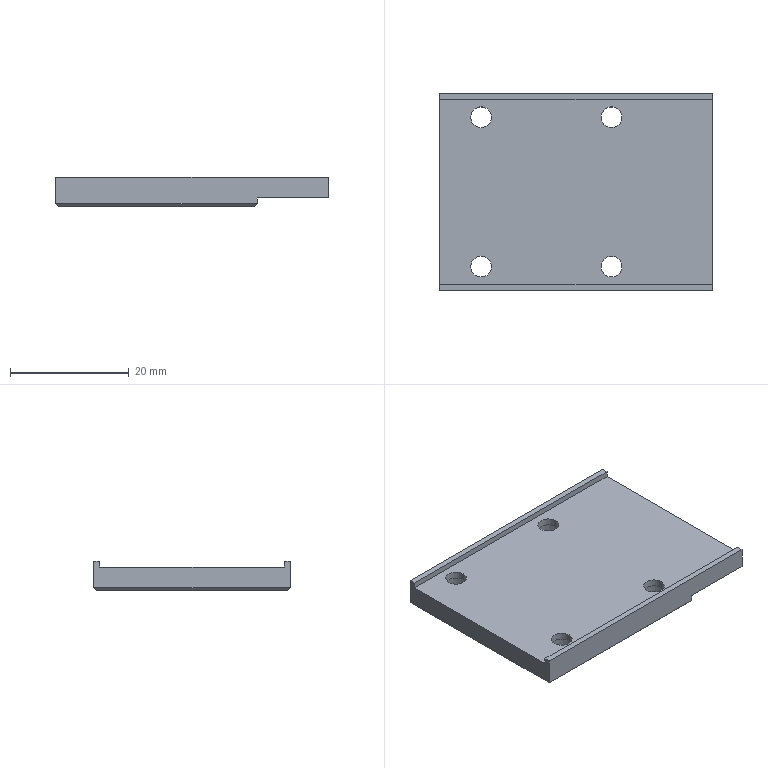Part | NX | 1 solid | 36 faces | box 46 x 33.2 x 5 mm | volume 5224 mm3 | plane 20 | cylinder 16 | commonest cylinder face diameters 3.5 x8 6 x8
STEP:
#1=CARTESIAN_POINT('',(0.,-32.2,4.5));
#2=VERTEX_POINT('',#1);
#3=CARTESIAN_POINT('',(46.,-32.2,4.5));
#4=VERTEX_POINT('',#3);
#5=CARTESIAN_POINT('',(0.,-32.2,4.5));
#6=DIRECTION('',(1.,0.,0.));
#7=VECTOR('',#6,1000.);
#8=LINE('',#5,#7);
#9=EDGE_CURVE('',#2,#4,#8,.T.);
#10=ORIENTED_EDGE('',*,*,#9,.T.);
#11=CARTESIAN_POINT('',(46.,-1.,4.5));
#12=VERTEX_POINT('',#11);
#13=CARTESIAN_POINT('',(46.,0.,4.5));
#14=DIRECTION('',(0.,-1.,0.));
#15=VECTOR('',#14,1000.);
#16=LINE('',#13,#15);
#17=EDGE_CURVE('',#12,#4,#16,.T.);
#18=ORIENTED_EDGE('',*,*,#17,.F.);
#19=CARTESIAN_POINT('',(0.,-1.,4.5));
#20=VERTEX_POINT('',#19);
#21=CARTESIAN_POINT('',(0.,-1.,4.5));
#22=DIRECTION('',(-1.,0.,0.));
#23=VECTOR('',#22,1000.);
#24=LINE('',#21,#23);
#25=EDGE_CURVE('',#12,#20,#24,.T.);
#26=ORIENTED_EDGE('',*,*,#25,.T.);
#27=CARTESIAN_POINT('',(0.,0.,4.5));
#28=DIRECTION('',(0.,1.,0.));
#29=VECTOR('',#28,1000.);
#30=LINE('',#27,#29);
#31=EDGE_CURVE('',#2,#20,#30,.T.);
#32=ORIENTED_EDGE('',*,*,#31,.F.);
#33=EDGE_LOOP('',(#10,#18,#26,#32));
#34=FACE_BOUND('',#33,.T.);
#35=CARTESIAN_POINT('',(8.75,-29.2,4.5));
#36=VERTEX_POINT('',#35);
#37=CARTESIAN_POINT('',(5.25,-29.2,4.5));
#38=VERTEX_POINT('',#37);
#39=CARTESIAN_POINT('',(7.,-29.2,4.5));
#40=DIRECTION('',(0.,0.,-1.));
#41=DIRECTION('',(1.,0.,0.));
#42=AXIS2_PLACEMENT_3D('',#39,#40,#41);
#43=CIRCLE('',#42,1.75);
#44=EDGE_CURVE('',#36,#38,#43,.T.);
#45=ORIENTED_EDGE('',*,*,#44,.T.);
#46=CARTESIAN_POINT('',(7.,-29.2,4.5));
#47=DIRECTION('',(0.,0.,-1.));
#48=DIRECTION('',(1.,0.,0.));
#49=AXIS2_PLACEMENT_3D('',#46,#47,#48);
#50=CIRCLE('',#49,1.75);
#51=EDGE_CURVE('',#38,#36,#50,.T.);
#52=ORIENTED_EDGE('',*,*,#51,.T.);
#53=EDGE_LOOP('',(#45,#52));
#54=FACE_BOUND('',#53,.T.);
#55=CARTESIAN_POINT('',(30.75,-4.,4.5));
#56=VERTEX_POINT('',#55);
#57=CARTESIAN_POINT('',(27.25,-4.,4.5));
#58=VERTEX_POINT('',#57);
#59=CARTESIAN_POINT('',(29.,-4.,4.5));
#60=DIRECTION('',(0.,0.,-1.));
#61=DIRECTION('',(1.,0.,0.));
#62=AXIS2_PLACEMENT_3D('',#59,#60,#61);
#63=CIRCLE('',#62,1.75);
#64=EDGE_CURVE('',#56,#58,#63,.T.);
#65=ORIENTED_EDGE('',*,*,#64,.T.);
#66=CARTESIAN_POINT('',(29.,-4.,4.5));
#67=DIRECTION('',(0.,0.,-1.));
#68=DIRECTION('',(1.,0.,0.));
#69=AXIS2_PLACEMENT_3D('',#66,#67,#68);
#70=CIRCLE('',#69,1.75);
#71=EDGE_CURVE('',#58,#56,#70,.T.);
#72=ORIENTED_EDGE('',*,*,#71,.T.);
#73=EDGE_LOOP('',(#65,#72));
#74=FACE_BOUND('',#73,.T.);
#75=CARTESIAN_POINT('',(27.25,-29.2,4.5));
#76=VERTEX_POINT('',#75);
#77=CARTESIAN_POINT('',(30.75,-29.2,4.5));
#78=VERTEX_POINT('',#77);
#79=CARTESIAN_POINT('',(29.,-29.2,4.5));
#80=DIRECTION('',(0.,0.,-1.));
#81=DIRECTION('',(1.,0.,0.));
#82=AXIS2_PLACEMENT_3D('',#79,#80,#81);
#83=CIRCLE('',#82,1.75);
#84=EDGE_CURVE('',#76,#78,#83,.T.);
#85=ORIENTED_EDGE('',*,*,#84,.T.);
#86=CARTESIAN_POINT('',(29.,-29.2,4.5));
#87=DIRECTION('',(0.,0.,-1.));
#88=DIRECTION('',(1.,0.,0.));
#89=AXIS2_PLACEMENT_3D('',#86,#87,#88);
#90=CIRCLE('',#89,1.75);
#91=EDGE_CURVE('',#78,#76,#90,.T.);
#92=ORIENTED_EDGE('',*,*,#91,.T.);
#93=EDGE_LOOP('',(#85,#92));
#94=FACE_BOUND('',#93,.T.);
#95=CARTESIAN_POINT('',(8.75,-4.,4.5));
#96=VERTEX_POINT('',#95);
#97=CARTESIAN_POINT('',(5.25,-4.,4.5));
#98=VERTEX_POINT('',#97);
#99=CARTESIAN_POINT('',(7.,-4.,4.5));
#100=DIRECTION('',(0.,0.,-1.));
#101=DIRECTION('',(1.,0.,0.));
#102=AXIS2_PLACEMENT_3D('',#99,#100,#101);
#103=CIRCLE('',#102,1.75);
#104=EDGE_CURVE('',#96,#98,#103,.T.);
#105=ORIENTED_EDGE('',*,*,#104,.T.);
#106=CARTESIAN_POINT('',(7.,-4.,4.5));
#107=DIRECTION('',(0.,0.,-1.));
#108=DIRECTION('',(1.,0.,0.));
#109=AXIS2_PLACEMENT_3D('',#106,#107,#108);
#110=CIRCLE('',#109,1.75);
#111=EDGE_CURVE('',#98,#96,#110,.T.);
#112=ORIENTED_EDGE('',*,*,#111,.T.);
#113=EDGE_LOOP('',(#105,#112));
#114=FACE_BOUND('',#113,.T.);
#115=CARTESIAN_POINT('',(0.,0.,4.5));
#116=DIRECTION('',(0.,0.,1.));
#117=DIRECTION('',(1.,0.,0.));
#118=AXIS2_PLACEMENT_3D('',#115,#116,#117);
#119=PLANE('',#118);
#120=ADVANCED_FACE('',(#34,#54,#74,#94,#114),#119,.T.);
#121=CARTESIAN_POINT('',(34.,0.,1.));
#122=VERTEX_POINT('',#121);
#123=CARTESIAN_POINT('',(34.,-33.2,1.));
#124=VERTEX_POINT('',#123);
#125=CARTESIAN_POINT('',(34.,0.,1.));
#126=DIRECTION('',(0.,-1.,0.));
#127=VECTOR('',#126,1000.);
#128=LINE('',#125,#127);
#129=EDGE_CURVE('',#122,#124,#128,.T.);
#130=ORIENTED_EDGE('',*,*,#129,.F.);
#131=CARTESIAN_POINT('',(34.,0.,2.));
#132=VERTEX_POINT('',#131);
#133=CARTESIAN_POINT('',(34.,0.,0.));
#134=DIRECTION('',(0.,0.,1.));
#135=VECTOR('',#134,1000.);
#136=LINE('',#133,#135);
#137=EDGE_CURVE('',#122,#132,#136,.T.);
#138=ORIENTED_EDGE('',*,*,#137,.T.);
#139=CARTESIAN_POINT('',(34.,-33.2,2.));
#140=VERTEX_POINT('',#139);
#141=CARTESIAN_POINT('',(34.,0.,2.));
#142=DIRECTION('',(0.,-1.,0.));
#143=VECTOR('',#142,1000.);
#144=LINE('',#141,#143);
#145=EDGE_CURVE('',#132,#140,#144,.T.);
#146=ORIENTED_EDGE('',*,*,#145,.T.);
#147=CARTESIAN_POINT('',(34.,-33.2,0.));
#148=DIRECTION('',(0.,0.,1.));
#149=VECTOR('',#148,1000.);
#150=LINE('',#147,#149);
#151=EDGE_CURVE('',#124,#140,#150,.T.);
#152=ORIENTED_EDGE('',*,*,#151,.F.);
#153=EDGE_LOOP('',(#130,#138,#146,#152));
#154=FACE_BOUND('',#153,.T.);
#155=CARTESIAN_POINT('',(34.,0.,0.));
#156=DIRECTION('',(-1.,0.,0.));
#157=DIRECTION('',(0.,0.,1.));
#158=AXIS2_PLACEMENT_3D('',#155,#156,#157);
#159=PLANE('',#158);
#160=ADVANCED_FACE('',(#154),#159,.F.);
#161=CARTESIAN_POINT('',(0.,-33.2,5.5));
#162=VERTEX_POINT('',#161);
#163=CARTESIAN_POINT('',(0.,-33.2,1.));
#164=VERTEX_POINT('',#163);
#165=CARTESIAN_POINT('',(0.,-33.2,0.));
#166=DIRECTION('',(0.,0.,-1.));
#167=VECTOR('',#166,1000.);
#168=LINE('',#165,#167);
#169=EDGE_CURVE('',#162,#164,#168,.T.);
#170=ORIENTED_EDGE('',*,*,#169,.T.);
#171=CARTESIAN_POINT('',(0.,-33.2,1.));
#172=DIRECTION('',(1.,0.,0.));
#173=VECTOR('',#172,1000.);
#174=LINE('',#171,#173);
#175=EDGE_CURVE('',#164,#124,#174,.T.);
#176=ORIENTED_EDGE('',*,*,#175,.T.);
#177=ORIENTED_EDGE('',*,*,#151,.T.);
#178=CARTESIAN_POINT('',(46.,-33.2,2.));
#179=VERTEX_POINT('',#178);
#180=CARTESIAN_POINT('',(0.,-33.2,2.));
#181=DIRECTION('',(1.,0.,0.));
#182=VECTOR('',#181,1000.);
#183=LINE('',#180,#182);
#184=EDGE_CURVE('',#140,#179,#183,.T.);
#185=ORIENTED_EDGE('',*,*,#184,.T.);
#186=CARTESIAN_POINT('',(46.,-33.2,5.5));
#187=VERTEX_POINT('',#186);
#188=CARTESIAN_POINT('',(46.,-33.2,0.));
#189=DIRECTION('',(0.,0.,-1.));
#190=VECTOR('',#189,1000.);
#191=LINE('',#188,#190);
#192=EDGE_CURVE('',#187,#179,#191,.T.);
#193=ORIENTED_EDGE('',*,*,#192,.F.);
#194=CARTESIAN_POINT('',(0.,-33.2,5.5));
#195=DIRECTION('',(1.,0.,0.));
#196=VECTOR('',#195,1000.);
#197=LINE('',#194,#196);
#198=EDGE_CURVE('',#162,#187,#197,.T.);
#199=ORIENTED_EDGE('',*,*,#198,.F.);
#200=EDGE_LOOP('',(#170,#176,#177,#185,#193,#199));
#201=FACE_BOUND('',#200,.T.);
#202=CARTESIAN_POINT('',(0.,-33.2,0.));
#203=DIRECTION('',(0.,-1.,0.));
#204=DIRECTION('',(0.,0.,-1.));
#205=AXIS2_PLACEMENT_3D('',#202,#203,#204);
#206=PLANE('',#205);
#207=ADVANCED_FACE('',(#201),#206,.T.);
#208=CARTESIAN_POINT('',(0.,0.,1.));
#209=VERTEX_POINT('',#208);
#210=CARTESIAN_POINT('',(0.,0.,5.5));
#211=VERTEX_POINT('',#210);
#212=CARTESIAN_POINT('',(0.,0.,0.));
#213=DIRECTION('',(0.,0.,1.));
#214=VECTOR('',#213,1000.);
#215=LINE('',#212,#214);
#216=EDGE_CURVE('',#209,#211,#215,.T.);
#217=ORIENTED_EDGE('',*,*,#216,.F.);
#218=CARTESIAN_POINT('',(0.,0.,1.));
#219=DIRECTION('',(0.,-1.,0.));
#220=VECTOR('',#219,1000.);
#221=LINE('',#218,#220);
#222=EDGE_CURVE('',#209,#164,#221,.T.);
#223=ORIENTED_EDGE('',*,*,#222,.T.);
#224=ORIENTED_EDGE('',*,*,#169,.F.);
#225=CARTESIAN_POINT('',(0.,-32.2,5.5));
#226=VERTEX_POINT('',#225);
#227=CARTESIAN_POINT('',(0.,0.,5.5));
#228=DIRECTION('',(0.,-1.,0.));
#229=VECTOR('',#228,1000.);
#230=LINE('',#227,#229);
#231=EDGE_CURVE('',#226,#162,#230,.T.);
#232=ORIENTED_EDGE('',*,*,#231,.F.);
#233=CARTESIAN_POINT('',(0.,-32.2,0.));
#234=DIRECTION('',(0.,0.,1.));
#235=VECTOR('',#234,1000.);
#236=LINE('',#233,#235);
#237=EDGE_CURVE('',#2,#226,#236,.T.);
#238=ORIENTED_EDGE('',*,*,#237,.F.);
#239=ORIENTED_EDGE('',*,*,#31,.T.);
#240=CARTESIAN_POINT('',(0.,-1.,5.5));
#241=VERTEX_POINT('',#240);
#242=CARTESIAN_POINT('',(0.,-1.,0.));
#243=DIRECTION('',(0.,0.,-1.));
#244=VECTOR('',#243,1000.);
#245=LINE('',#242,#244);
#246=EDGE_CURVE('',#241,#20,#245,.T.);
#247=ORIENTED_EDGE('',*,*,#246,.F.);
#248=CARTESIAN_POINT('',(0.,0.,5.5));
#249=DIRECTION('',(0.,-1.,0.));
#250=VECTOR('',#249,1000.);
#251=LINE('',#248,#250);
#252=EDGE_CURVE('',#211,#241,#251,.T.);
#253=ORIENTED_EDGE('',*,*,#252,.F.);
#254=EDGE_LOOP('',(#217,#223,#224,#232,#238,#239,#247,#253));
#255=FACE_BOUND('',#254,.T.);
#256=CARTESIAN_POINT('',(0.,0.,0.));
#257=DIRECTION('',(-1.,0.,0.));
#258=DIRECTION('',(0.,0.,1.));
#259=AXIS2_PLACEMENT_3D('',#256,#257,#258);
#260=PLANE('',#259);
#261=ADVANCED_FACE('',(#255),#260,.T.);
#262=ORIENTED_EDGE('',*,*,#137,.F.);
#263=CARTESIAN_POINT('',(0.,0.,1.));
#264=DIRECTION('',(1.,0.,0.));
#265=VECTOR('',#264,1000.);
#266=LINE('',#263,#265);
#267=EDGE_CURVE('',#209,#122,#266,.T.);
#268=ORIENTED_EDGE('',*,*,#267,.F.);
#269=ORIENTED_EDGE('',*,*,#216,.T.);
#270=CARTESIAN_POINT('',(46.,0.,5.5));
#271=VERTEX_POINT('',#270);
#272=CARTESIAN_POINT('',(0.,0.,5.5));
#273=DIRECTION('',(-1.,0.,0.));
#274=VECTOR('',#273,1000.);
#275=LINE('',#272,#274);
#276=EDGE_CURVE('',#271,#211,#275,.T.);
#277=ORIENTED_EDGE('',*,*,#276,.F.);
#278=CARTESIAN_POINT('',(46.,0.,2.));
#279=VERTEX_POINT('',#278);
#280=CARTESIAN_POINT('',(46.,0.,0.));
#281=DIRECTION('',(0.,0.,1.));
#282=VECTOR('',#281,1000.);
#283=LINE('',#280,#282);
#284=EDGE_CURVE('',#279,#271,#283,.T.);
#285=ORIENTED_EDGE('',*,*,#284,.F.);
#286=CARTESIAN_POINT('',(0.,0.,2.));
#287=DIRECTION('',(-1.,0.,0.));
#288=VECTOR('',#287,1000.);
#289=LINE('',#286,#288);
#290=EDGE_CURVE('',#279,#132,#289,.T.);
#291=ORIENTED_EDGE('',*,*,#290,.T.);
#292=EDGE_LOOP('',(#262,#268,#269,#277,#285,#291));
#293=FACE_BOUND('',#292,.T.);
#294=CARTESIAN_POINT('',(46.,0.,0.));
#295=DIRECTION('',(0.,1.,0.));
#296=DIRECTION('',(1.,0.,0.));
#297=AXIS2_PLACEMENT_3D('',#294,#295,#296);
#298=PLANE('',#297);
#299=ADVANCED_FACE('',(#293),#298,.T.);
#300=ORIENTED_EDGE('',*,*,#184,.F.);
#301=ORIENTED_EDGE('',*,*,#145,.F.);
#302=ORIENTED_EDGE('',*,*,#290,.F.);
#303=CARTESIAN_POINT('',(46.,0.,2.));
#304=DIRECTION('',(0.,-1.,0.));
#305=VECTOR('',#304,1000.);
#306=LINE('',#303,#305);
#307=EDGE_CURVE('',#279,#179,#306,.T.);
#308=ORIENTED_EDGE('',*,*,#307,.T.);
#309=EDGE_LOOP('',(#300,#301,#302,#308));
#310=FACE_BOUND('',#309,.T.);
#311=CARTESIAN_POINT('',(34.,0.,2.));
#312=DIRECTION('',(0.,0.,1.));
#313=DIRECTION('',(1.,0.,0.));
#314=AXIS2_PLACEMENT_3D('',#311,#312,#313);
#315=PLANE('',#314);
#316=ADVANCED_FACE('',(#310),#315,.F.);
#317=ORIENTED_EDGE('',*,*,#307,.F.);
#318=ORIENTED_EDGE('',*,*,#284,.T.);
#319=CARTESIAN_POINT('',(46.,-1.,5.5));
#320=VERTEX_POINT('',#319);
#321=CARTESIAN_POINT('',(46.,0.,5.5));
#322=DIRECTION('',(0.,-1.,0.));
#323=VECTOR('',#322,1000.);
#324=LINE('',#321,#323);
#325=EDGE_CURVE('',#271,#320,#324,.T.);
#326=ORIENTED_EDGE('',*,*,#325,.T.);
#327=CARTESIAN_POINT('',(46.,-1.,5.5));
#328=DIRECTION('',(0.,0.,-1.));
#329=VECTOR('',#328,1000.);
#330=LINE('',#327,#329);
#331=EDGE_CURVE('',#320,#12,#330,.T.);
#332=ORIENTED_EDGE('',*,*,#331,.T.);
#333=ORIENTED_EDGE('',*,*,#17,.T.);
#334=CARTESIAN_POINT('',(46.,-32.2,5.5));
#335=VERTEX_POINT('',#334);
#336=CARTESIAN_POINT('',(46.,-32.2,5.5));
#337=DIRECTION('',(0.,0.,-1.));
#338=VECTOR('',#337,1000.);
#339=LINE('',#336,#338);
#340=EDGE_CURVE('',#335,#4,#339,.T.);
#341=ORIENTED_EDGE('',*,*,#340,.F.);
#342=CARTESIAN_POINT('',(46.,-32.2,5.5));
#343=DIRECTION('',(0.,-1.,0.));
#344=VECTOR('',#343,1000.);
#345=LINE('',#342,#344);
#346=EDGE_CURVE('',#335,#187,#345,.T.);
#347=ORIENTED_EDGE('',*,*,#346,.T.);
#348=ORIENTED_EDGE('',*,*,#192,.T.);
#349=EDGE_LOOP('',(#317,#318,#326,#332,#333,#341,#347,#348));
#350=FACE_BOUND('',#349,.T.);
#351=CARTESIAN_POINT('',(46.,-33.2,0.));
#352=DIRECTION('',(1.,0.,0.));
#353=DIRECTION('',(0.,1.,0.));
#354=AXIS2_PLACEMENT_3D('',#351,#352,#353);
#355=PLANE('',#354);
#356=ADVANCED_FACE('',(#350),#355,.T.);
#357=ORIENTED_EDGE('',*,*,#346,.F.);
#358=CARTESIAN_POINT('',(0.,-32.2,5.5));
#359=DIRECTION('',(1.,0.,0.));
#360=VECTOR('',#359,1000.);
#361=LINE('',#358,#360);
#362=EDGE_CURVE('',#226,#335,#361,.T.);
#363=ORIENTED_EDGE('',*,*,#362,.F.);
#364=ORIENTED_EDGE('',*,*,#231,.T.);
#365=ORIENTED_EDGE('',*,*,#198,.T.);
#366=EDGE_LOOP('',(#357,#363,#364,#365));
#367=FACE_BOUND('',#366,.T.);
#368=CARTESIAN_POINT('',(0.,0.,5.5));
#369=DIRECTION('',(0.,0.,1.));
#370=DIRECTION('',(1.,0.,0.));
#371=AXIS2_PLACEMENT_3D('',#368,#369,#370);
#372=PLANE('',#371);
#373=ADVANCED_FACE('',(#367),#372,.T.);
#374=ORIENTED_EDGE('',*,*,#9,.F.);
#375=ORIENTED_EDGE('',*,*,#237,.T.);
#376=ORIENTED_EDGE('',*,*,#362,.T.);
#377=ORIENTED_EDGE('',*,*,#340,.T.);
#378=EDGE_LOOP('',(#374,#375,#376,#377));
#379=FACE_BOUND('',#378,.T.);
#380=CARTESIAN_POINT('',(46.,-32.2,4.5));
#381=DIRECTION('',(0.,1.,0.));
#382=DIRECTION('',(1.,0.,0.));
#383=AXIS2_PLACEMENT_3D('',#380,#381,#382);
#384=PLANE('',#383);
#385=ADVANCED_FACE('',(#379),#384,.T.);
#386=CARTESIAN_POINT('',(0.5,-0.5,0.5));
#387=VERTEX_POINT('',#386);
#388=CARTESIAN_POINT('',(0.5,-32.7,0.5));
#389=VERTEX_POINT('',#388);
#390=CARTESIAN_POINT('',(0.5,0.,0.5));
#391=DIRECTION('',(0.,-1.,0.));
#392=VECTOR('',#391,1000.);
#393=LINE('',#390,#392);
#394=EDGE_CURVE('',#387,#389,#393,.T.);
#395=ORIENTED_EDGE('',*,*,#394,.F.);
#396=CARTESIAN_POINT('',(33.5,-0.5,0.5));
#397=VERTEX_POINT('',#396);
#398=CARTESIAN_POINT('',(0.,-0.5,0.5));
#399=DIRECTION('',(1.,0.,0.));
#400=VECTOR('',#399,1000.);
#401=LINE('',#398,#400);
#402=EDGE_CURVE('',#387,#397,#401,.T.);
#403=ORIENTED_EDGE('',*,*,#402,.T.);
#404=CARTESIAN_POINT('',(33.5,-32.7,0.5));
#405=VERTEX_POINT('',#404);
#406=CARTESIAN_POINT('',(33.5,0.,0.5));
#407=DIRECTION('',(0.,1.,0.));
#408=VECTOR('',#407,1000.);
#409=LINE('',#406,#408);
#410=EDGE_CURVE('',#405,#397,#409,.T.);
#411=ORIENTED_EDGE('',*,*,#410,.F.);
#412=CARTESIAN_POINT('',(0.,-32.7,0.5));
#413=DIRECTION('',(1.,0.,0.));
#414=VECTOR('',#413,1000.);
#415=LINE('',#412,#414);
#416=EDGE_CURVE('',#389,#405,#415,.T.);
#417=ORIENTED_EDGE('',*,*,#416,.F.);
#418=EDGE_LOOP('',(#395,#403,#411,#417));
#419=FACE_BOUND('',#418,.T.);
#420=CARTESIAN_POINT('',(4.,-4.,0.5));
#421=VERTEX_POINT('',#420);
#422=CARTESIAN_POINT('',(10.,-4.,0.5));
#423=VERTEX_POINT('',#422);
#424=CARTESIAN_POINT('',(7.,-4.,0.5));
#425=DIRECTION('',(0.,0.,-1.));
#426=DIRECTION('',(1.,0.,0.));
#427=AXIS2_PLACEMENT_3D('',#424,#425,#426);
#428=CIRCLE('',#427,3.);
#429=EDGE_CURVE('',#421,#423,#428,.T.);
#430=ORIENTED_EDGE('',*,*,#429,.F.);
#431=CARTESIAN_POINT('',(7.,-4.,0.5));
#432=DIRECTION('',(0.,0.,-1.));
#433=DIRECTION('',(1.,0.,0.));
#434=AXIS2_PLACEMENT_3D('',#431,#432,#433);
#435=CIRCLE('',#434,3.);
#436=EDGE_CURVE('',#423,#421,#435,.T.);
#437=ORIENTED_EDGE('',*,*,#436,.F.);
#438=EDGE_LOOP('',(#430,#437));
#439=FACE_BOUND('',#438,.T.);
#440=CARTESIAN_POINT('',(4.,-29.2,0.5));
#441=VERTEX_POINT('',#440);
#442=CARTESIAN_POINT('',(10.,-29.2,0.5));
#443=VERTEX_POINT('',#442);
#444=CARTESIAN_POINT('',(7.,-29.2,0.5));
#445=DIRECTION('',(0.,0.,-1.));
#446=DIRECTION('',(1.,0.,0.));
#447=AXIS2_PLACEMENT_3D('',#444,#445,#446);
#448=CIRCLE('',#447,3.);
#449=EDGE_CURVE('',#441,#443,#448,.T.);
#450=ORIENTED_EDGE('',*,*,#449,.F.);
#451=CARTESIAN_POINT('',(7.,-29.2,0.5));
#452=DIRECTION('',(0.,0.,-1.));
#453=DIRECTION('',(1.,0.,0.));
#454=AXIS2_PLACEMENT_3D('',#451,#452,#453);
#455=CIRCLE('',#454,3.);
#456=EDGE_CURVE('',#443,#441,#455,.T.);
#457=ORIENTED_EDGE('',*,*,#456,.F.);
#458=EDGE_LOOP('',(#450,#457));
#459=FACE_BOUND('',#458,.T.);
#460=CARTESIAN_POINT('',(32.,-4.,0.5));
#461=VERTEX_POINT('',#460);
#462=CARTESIAN_POINT('',(26.,-4.,0.5));
#463=VERTEX_POINT('',#462);
#464=CARTESIAN_POINT('',(29.,-4.,0.5));
#465=DIRECTION('',(0.,0.,-1.));
#466=DIRECTION('',(1.,0.,0.));
#467=AXIS2_PLACEMENT_3D('',#464,#465,#466);
#468=CIRCLE('',#467,3.);
#469=EDGE_CURVE('',#461,#463,#468,.T.);
#470=ORIENTED_EDGE('',*,*,#469,.F.);
#471=CARTESIAN_POINT('',(29.,-4.,0.5));
#472=DIRECTION('',(0.,0.,-1.));
#473=DIRECTION('',(1.,0.,0.));
#474=AXIS2_PLACEMENT_3D('',#471,#472,#473);
#475=CIRCLE('',#474,3.);
#476=EDGE_CURVE('',#463,#461,#475,.T.);
#477=ORIENTED_EDGE('',*,*,#476,.F.);
#478=EDGE_LOOP('',(#470,#477));
#479=FACE_BOUND('',#478,.T.);
#480=CARTESIAN_POINT('',(26.,-29.2,0.5));
#481=VERTEX_POINT('',#480);
#482=CARTESIAN_POINT('',(32.,-29.2,0.5));
#483=VERTEX_POINT('',#482);
#484=CARTESIAN_POINT('',(29.,-29.2,0.5));
#485=DIRECTION('',(0.,0.,-1.));
#486=DIRECTION('',(1.,0.,0.));
#487=AXIS2_PLACEMENT_3D('',#484,#485,#486);
#488=CIRCLE('',#487,3.);
#489=EDGE_CURVE('',#481,#483,#488,.T.);
#490=ORIENTED_EDGE('',*,*,#489,.F.);
#491=CARTESIAN_POINT('',(29.,-29.2,0.5));
#492=DIRECTION('',(0.,0.,-1.));
#493=DIRECTION('',(1.,0.,0.));
#494=AXIS2_PLACEMENT_3D('',#491,#492,#493);
#495=CIRCLE('',#494,3.);
#496=EDGE_CURVE('',#483,#481,#495,.T.);
#497=ORIENTED_EDGE('',*,*,#496,.F.);
#498=EDGE_LOOP('',(#490,#497));
#499=FACE_BOUND('',#498,.T.);
#500=CARTESIAN_POINT('',(0.,0.,0.5));
#501=DIRECTION('',(0.,0.,1.));
#502=DIRECTION('',(1.,0.,0.));
#503=AXIS2_PLACEMENT_3D('',#500,#501,#502);
#504=PLANE('',#503);
#505=ADVANCED_FACE('',(#419,#439,#459,#479,#499),#504,.F.);
#506=ORIENTED_EDGE('',*,*,#25,.F.);
#507=ORIENTED_EDGE('',*,*,#331,.F.);
#508=CARTESIAN_POINT('',(46.,-1.,5.5));
#509=DIRECTION('',(-1.,0.,0.));
#510=VECTOR('',#509,1000.);
#511=LINE('',#508,#510);
#512=EDGE_CURVE('',#320,#241,#511,.T.);
#513=ORIENTED_EDGE('',*,*,#512,.T.);
#514=ORIENTED_EDGE('',*,*,#246,.T.);
#515=EDGE_LOOP('',(#506,#507,#513,#514));
#516=FACE_BOUND('',#515,.T.);
#517=CARTESIAN_POINT('',(0.,-1.,4.5));
#518=DIRECTION('',(0.,-1.,0.));
#519=DIRECTION('',(0.,0.,-1.));
#520=AXIS2_PLACEMENT_3D('',#517,#518,#519);
#521=PLANE('',#520);
#522=ADVANCED_FACE('',(#516),#521,.T.);
#523=ORIENTED_EDGE('',*,*,#276,.T.);
#524=ORIENTED_EDGE('',*,*,#252,.T.);
#525=ORIENTED_EDGE('',*,*,#512,.F.);
#526=ORIENTED_EDGE('',*,*,#325,.F.);
#527=EDGE_LOOP('',(#523,#524,#525,#526));
#528=FACE_BOUND('',#527,.T.);
#529=CARTESIAN_POINT('',(0.,0.,5.5));
#530=DIRECTION('',(0.,0.,1.));
#531=DIRECTION('',(1.,0.,0.));
#532=AXIS2_PLACEMENT_3D('',#529,#530,#531);
#533=PLANE('',#532);
#534=ADVANCED_FACE('',(#528),#533,.T.);
#535=ORIENTED_EDGE('',*,*,#44,.F.);
#536=CARTESIAN_POINT('',(8.75,-29.2,3.3));
#537=VERTEX_POINT('',#536);
#538=CARTESIAN_POINT('',(8.75,-29.2,5.225));
#539=DIRECTION('',(0.,0.,-1.));
#540=VECTOR('',#539,1000.);
#541=LINE('',#538,#540);
#542=EDGE_CURVE('',#36,#537,#541,.T.);
#543=ORIENTED_EDGE('',*,*,#542,.T.);
#544=CARTESIAN_POINT('',(5.25,-29.2,3.3));
#545=VERTEX_POINT('',#544);
#546=CARTESIAN_POINT('',(7.,-29.2,3.3));
#547=DIRECTION('',(0.,0.,-1.));
#548=DIRECTION('',(1.,0.,0.));
#549=AXIS2_PLACEMENT_3D('',#546,#547,#548);
#550=CIRCLE('',#549,1.75);
#551=EDGE_CURVE('',#537,#545,#550,.T.);
#552=ORIENTED_EDGE('',*,*,#551,.T.);
#553=CARTESIAN_POINT('',(5.25,-29.2,5.225));
#554=DIRECTION('',(0.,0.,-1.));
#555=VECTOR('',#554,1000.);
#556=LINE('',#553,#555);
#557=EDGE_CURVE('',#38,#545,#556,.T.);
#558=ORIENTED_EDGE('',*,*,#557,.F.);
#559=EDGE_LOOP('',(#535,#543,#552,#558));
#560=FACE_BOUND('',#559,.T.);
#561=CARTESIAN_POINT('',(7.,-29.2,5.225));
#562=DIRECTION('',(0.,0.,-1.));
#563=DIRECTION('',(1.,0.,0.));
#564=AXIS2_PLACEMENT_3D('',#561,#562,#563);
#565=CYLINDRICAL_SURFACE('',#564,1.75);
#566=ADVANCED_FACE('',(#560),#565,.F.);
#567=ORIENTED_EDGE('',*,*,#104,.F.);
#568=CARTESIAN_POINT('',(8.75,-4.,3.3));
#569=VERTEX_POINT('',#568);
#570=CARTESIAN_POINT('',(8.75,-4.,6.353));
#571=DIRECTION('',(0.,0.,-1.));
#572=VECTOR('',#571,1000.);
#573=LINE('',#570,#572);
#574=EDGE_CURVE('',#96,#569,#573,.T.);
#575=ORIENTED_EDGE('',*,*,#574,.T.);
#576=CARTESIAN_POINT('',(5.25,-4.,3.3));
#577=VERTEX_POINT('',#576);
#578=CARTESIAN_POINT('',(7.,-4.,3.3));
#579=DIRECTION('',(0.,0.,-1.));
#580=DIRECTION('',(1.,0.,0.));
#581=AXIS2_PLACEMENT_3D('',#578,#579,#580);
#582=CIRCLE('',#581,1.75);
#583=EDGE_CURVE('',#569,#577,#582,.T.);
#584=ORIENTED_EDGE('',*,*,#583,.T.);
#585=CARTESIAN_POINT('',(5.25,-4.,6.353));
#586=DIRECTION('',(0.,0.,-1.));
#587=VECTOR('',#586,1000.);
#588=LINE('',#585,#587);
#589=EDGE_CURVE('',#98,#577,#588,.T.);
#590=ORIENTED_EDGE('',*,*,#589,.F.);
#591=EDGE_LOOP('',(#567,#575,#584,#590));
#592=FACE_BOUND('',#591,.T.);
#593=CARTESIAN_POINT('',(7.,-4.,6.353));
#594=DIRECTION('',(0.,0.,-1.));
#595=DIRECTION('',(1.,0.,0.));
#596=AXIS2_PLACEMENT_3D('',#593,#594,#595);
#597=CYLINDRICAL_SURFACE('',#596,1.75);
#598=ADVANCED_FACE('',(#592),#597,.F.);
#599=CARTESIAN_POINT('',(26.,-4.,3.3));
#600=VERTEX_POINT('',#599);
#601=CARTESIAN_POINT('',(32.,-4.,3.3));
#602=VERTEX_POINT('',#601);
#603=CARTESIAN_POINT('',(29.,-4.,3.3));
#604=DIRECTION('',(0.,0.,-1.));
#605=DIRECTION('',(1.,0.,0.));
#606=AXIS2_PLACEMENT_3D('',#603,#604,#605);
#607=CIRCLE('',#606,3.);
#608=EDGE_CURVE('',#600,#602,#607,.T.);
#609=ORIENTED_EDGE('',*,*,#608,.T.);
#610=CARTESIAN_POINT('',(29.,-4.,3.3));
#611=DIRECTION('',(0.,0.,-1.));
#612=DIRECTION('',(1.,0.,0.));
#613=AXIS2_PLACEMENT_3D('',#610,#611,#612);
#614=CIRCLE('',#613,3.);
#615=EDGE_CURVE('',#602,#600,#614,.T.);
#616=ORIENTED_EDGE('',*,*,#615,.T.);
#617=EDGE_LOOP('',(#609,#616));
#618=FACE_BOUND('',#617,.T.);
#619=CARTESIAN_POINT('',(27.25,-4.,3.3));
#620=VERTEX_POINT('',#619);
#621=CARTESIAN_POINT('',(30.75,-4.,3.3));
#622=VERTEX_POINT('',#621);
#623=CARTESIAN_POINT('',(29.,-4.,3.3));
#624=DIRECTION('',(0.,0.,-1.));
#625=DIRECTION('',(1.,0.,0.));
#626=AXIS2_PLACEMENT_3D('',#623,#624,#625);
#627=CIRCLE('',#626,1.75);
#628=EDGE_CURVE('',#620,#622,#627,.T.);
#629=ORIENTED_EDGE('',*,*,#628,.F.);
#630=CARTESIAN_POINT('',(29.,-4.,3.3));
#631=DIRECTION('',(0.,0.,-1.));
#632=DIRECTION('',(1.,0.,0.));
#633=AXIS2_PLACEMENT_3D('',#630,#631,#632);
#634=CIRCLE('',#633,1.75);
#635=EDGE_CURVE('',#622,#620,#634,.T.);
#636=ORIENTED_EDGE('',*,*,#635,.F.);
#637=EDGE_LOOP('',(#629,#636));
#638=FACE_BOUND('',#637,.T.);
#639=CARTESIAN_POINT('',(7.,-4.,3.3));
#640=DIRECTION('',(0.,0.,-1.));
#641=DIRECTION('',(0.,-1.,0.));
#642=AXIS2_PLACEMENT_3D('',#639,#640,#641);
#643=PLANE('',#642);
#644=ADVANCED_FACE('',(#618,#638),#643,.T.);
#645=CARTESIAN_POINT('',(10.,-29.2,3.3));
#646=VERTEX_POINT('',#645);
#647=CARTESIAN_POINT('',(4.,-29.2,3.3));
#648=VERTEX_POINT('',#647);
#649=CARTESIAN_POINT('',(7.,-29.2,3.3));
#650=DIRECTION('',(0.,0.,-1.));
#651=DIRECTION('',(1.,0.,0.));
#652=AXIS2_PLACEMENT_3D('',#649,#650,#651);
#653=CIRCLE('',#652,3.);
#654=EDGE_CURVE('',#646,#648,#653,.T.);
#655=ORIENTED_EDGE('',*,*,#654,.F.);
#656=CARTESIAN_POINT('',(10.,-29.2,5.225));
#657=DIRECTION('',(0.,0.,-1.));
#658=VECTOR('',#657,1000.);
#659=LINE('',#656,#658);
#660=EDGE_CURVE('',#646,#443,#659,.T.);
#661=ORIENTED_EDGE('',*,*,#660,.T.);
#662=ORIENTED_EDGE('',*,*,#456,.T.);
#663=CARTESIAN_POINT('',(4.,-29.2,5.225));
#664=DIRECTION('',(0.,0.,-1.));
#665=VECTOR('',#664,1000.);
#666=LINE('',#663,#665);
#667=EDGE_CURVE('',#648,#441,#666,.T.);
#668=ORIENTED_EDGE('',*,*,#667,.F.);
#669=EDGE_LOOP('',(#655,#661,#662,#668));
#670=FACE_BOUND('',#669,.T.);
#671=CARTESIAN_POINT('',(7.,-29.2,5.225));
#672=DIRECTION('',(0.,0.,-1.));
#673=DIRECTION('',(1.,0.,0.));
#674=AXIS2_PLACEMENT_3D('',#671,#672,#673);
#675=CYLINDRICAL_SURFACE('',#674,3.);
#676=ADVANCED_FACE('',(#670),#675,.F.);
#677=ORIENTED_EDGE('',*,*,#654,.T.);
#678=CARTESIAN_POINT('',(7.,-29.2,3.3));
#679=DIRECTION('',(0.,0.,-1.));
#680=DIRECTION('',(1.,0.,0.));
#681=AXIS2_PLACEMENT_3D('',#678,#679,#680);
#682=CIRCLE('',#681,3.);
#683=EDGE_CURVE('',#648,#646,#682,.T.);
#684=ORIENTED_EDGE('',*,*,#683,.T.);
#685=EDGE_LOOP('',(#677,#684));
#686=FACE_BOUND('',#685,.T.);
#687=CARTESIAN_POINT('',(7.,-29.2,3.3));
#688=DIRECTION('',(0.,0.,-1.));
#689=DIRECTION('',(1.,0.,0.));
#690=AXIS2_PLACEMENT_3D('',#687,#688,#689);
#691=CIRCLE('',#690,1.75);
#692=EDGE_CURVE('',#545,#537,#691,.T.);
#693=ORIENTED_EDGE('',*,*,#692,.F.);
#694=ORIENTED_EDGE('',*,*,#551,.F.);
#695=EDGE_LOOP('',(#693,#694));
#696=FACE_BOUND('',#695,.T.);
#697=CARTESIAN_POINT('',(7.,-4.,3.3));
#698=DIRECTION('',(0.,0.,-1.));
#699=DIRECTION('',(0.,-1.,0.));
#700=AXIS2_PLACEMENT_3D('',#697,#698,#699);
#701=PLANE('',#700);
#702=ADVANCED_FACE('',(#686,#696),#701,.T.);
#703=ORIENTED_EDGE('',*,*,#64,.F.);
#704=CARTESIAN_POINT('',(30.75,-4.,6.38));
#705=DIRECTION('',(0.,0.,-1.));
#706=VECTOR('',#705,1000.);
#707=LINE('',#704,#706);
#708=EDGE_CURVE('',#56,#622,#707,.T.);
#709=ORIENTED_EDGE('',*,*,#708,.T.);
#710=ORIENTED_EDGE('',*,*,#635,.T.);
#711=CARTESIAN_POINT('',(27.25,-4.,6.38));
#712=DIRECTION('',(0.,0.,-1.));
#713=VECTOR('',#712,1000.);
#714=LINE('',#711,#713);
#715=EDGE_CURVE('',#58,#620,#714,.T.);
#716=ORIENTED_EDGE('',*,*,#715,.F.);
#717=EDGE_LOOP('',(#703,#709,#710,#716));
#718=FACE_BOUND('',#717,.T.);
#719=CARTESIAN_POINT('',(29.,-4.,6.38));
#720=DIRECTION('',(0.,0.,-1.));
#721=DIRECTION('',(1.,0.,0.));
#722=AXIS2_PLACEMENT_3D('',#719,#720,#721);
#723=CYLINDRICAL_SURFACE('',#722,1.75);
#724=ADVANCED_FACE('',(#718),#723,.F.);
#725=CARTESIAN_POINT('',(4.,-4.,3.3));
#726=VERTEX_POINT('',#725);
#727=CARTESIAN_POINT('',(10.,-4.,3.3));
#728=VERTEX_POINT('',#727);
#729=CARTESIAN_POINT('',(7.,-4.,3.3));
#730=DIRECTION('',(0.,0.,-1.));
#731=DIRECTION('',(1.,0.,0.));
#732=AXIS2_PLACEMENT_3D('',#729,#730,#731);
#733=CIRCLE('',#732,3.);
#734=EDGE_CURVE('',#726,#728,#733,.T.);
#735=ORIENTED_EDGE('',*,*,#734,.T.);
#736=CARTESIAN_POINT('',(7.,-4.,3.3));
#737=DIRECTION('',(0.,0.,-1.));
#738=DIRECTION('',(1.,0.,0.));
#739=AXIS2_PLACEMENT_3D('',#736,#737,#738);
#740=CIRCLE('',#739,3.);
#741=EDGE_CURVE('',#728,#726,#740,.T.);
#742=ORIENTED_EDGE('',*,*,#741,.T.);
#743=EDGE_LOOP('',(#735,#742));
#744=FACE_BOUND('',#743,.T.);
#745=ORIENTED_EDGE('',*,*,#583,.F.);
#746=CARTESIAN_POINT('',(7.,-4.,3.3));
#747=DIRECTION('',(0.,0.,-1.));
#748=DIRECTION('',(1.,0.,0.));
#749=AXIS2_PLACEMENT_3D('',#746,#747,#748);
#750=CIRCLE('',#749,1.75);
#751=EDGE_CURVE('',#577,#569,#750,.T.);
#752=ORIENTED_EDGE('',*,*,#751,.F.);
#753=EDGE_LOOP('',(#745,#752));
#754=FACE_BOUND('',#753,.T.);
#755=CARTESIAN_POINT('',(7.,-4.,3.3));
#756=DIRECTION('',(0.,0.,-1.));
#757=DIRECTION('',(0.,-1.,0.));
#758=AXIS2_PLACEMENT_3D('',#755,#756,#757);
#759=PLANE('',#758);
#760=ADVANCED_FACE('',(#744,#754),#759,.T.);
#761=CARTESIAN_POINT('',(26.,-29.2,3.3));
#762=VERTEX_POINT('',#761);
#763=CARTESIAN_POINT('',(32.,-29.2,3.3));
#764=VERTEX_POINT('',#763);
#765=CARTESIAN_POINT('',(29.,-29.2,3.3));
#766=DIRECTION('',(0.,0.,-1.));
#767=DIRECTION('',(1.,0.,0.));
#768=AXIS2_PLACEMENT_3D('',#765,#766,#767);
#769=CIRCLE('',#768,3.);
#770=EDGE_CURVE('',#762,#764,#769,.T.);
#771=ORIENTED_EDGE('',*,*,#770,.T.);
#772=CARTESIAN_POINT('',(29.,-29.2,3.3));
#773=DIRECTION('',(0.,0.,-1.));
#774=DIRECTION('',(1.,0.,0.));
#775=AXIS2_PLACEMENT_3D('',#772,#773,#774);
#776=CIRCLE('',#775,3.);
#777=EDGE_CURVE('',#764,#762,#776,.T.);
#778=ORIENTED_EDGE('',*,*,#777,.T.);
#779=EDGE_LOOP('',(#771,#778));
#780=FACE_BOUND('',#779,.T.);
#781=CARTESIAN_POINT('',(30.75,-29.2,3.3));
#782=VERTEX_POINT('',#781);
#783=CARTESIAN_POINT('',(27.25,-29.2,3.3));
#784=VERTEX_POINT('',#783);
#785=CARTESIAN_POINT('',(29.,-29.2,3.3));
#786=DIRECTION('',(0.,0.,-1.));
#787=DIRECTION('',(1.,0.,0.));
#788=AXIS2_PLACEMENT_3D('',#785,#786,#787);
#789=CIRCLE('',#788,1.75);
#790=EDGE_CURVE('',#782,#784,#789,.T.);
#791=ORIENTED_EDGE('',*,*,#790,.F.);
#792=CARTESIAN_POINT('',(29.,-29.2,3.3));
#793=DIRECTION('',(0.,0.,-1.));
#794=DIRECTION('',(1.,0.,0.));
#795=AXIS2_PLACEMENT_3D('',#792,#793,#794);
#796=CIRCLE('',#795,1.75);
#797=EDGE_CURVE('',#784,#782,#796,.T.);
#798=ORIENTED_EDGE('',*,*,#797,.F.);
#799=EDGE_LOOP('',(#791,#798));
#800=FACE_BOUND('',#799,.T.);
#801=CARTESIAN_POINT('',(7.,-4.,3.3));
#802=DIRECTION('',(0.,0.,-1.));
#803=DIRECTION('',(0.,-1.,0.));
#804=AXIS2_PLACEMENT_3D('',#801,#802,#803);
#805=PLANE('',#804);
#806=ADVANCED_FACE('',(#780,#800),#805,.T.);
#807=ORIENTED_EDGE('',*,*,#469,.T.);
#808=CARTESIAN_POINT('',(26.,-4.,6.38));
#809=DIRECTION('',(0.,0.,-1.));
#810=VECTOR('',#809,1000.);
#811=LINE('',#808,#810);
#812=EDGE_CURVE('',#463,#600,#811,.F.);
#813=ORIENTED_EDGE('',*,*,#812,.T.);
#814=ORIENTED_EDGE('',*,*,#615,.F.);
#815=CARTESIAN_POINT('',(32.,-4.,6.38));
#816=DIRECTION('',(0.,0.,-1.));
#817=VECTOR('',#816,1000.);
#818=LINE('',#815,#817);
#819=EDGE_CURVE('',#461,#602,#818,.F.);
#820=ORIENTED_EDGE('',*,*,#819,.F.);
#821=EDGE_LOOP('',(#807,#813,#814,#820));
#822=FACE_BOUND('',#821,.T.);
#823=CARTESIAN_POINT('',(29.,-4.,6.38));
#824=DIRECTION('',(0.,0.,-1.));
#825=DIRECTION('',(1.,0.,0.));
#826=AXIS2_PLACEMENT_3D('',#823,#824,#825);
#827=CYLINDRICAL_SURFACE('',#826,3.);
#828=ADVANCED_FACE('',(#822),#827,.F.);
#829=ORIENTED_EDGE('',*,*,#734,.F.);
#830=CARTESIAN_POINT('',(4.,-4.,6.353));
#831=DIRECTION('',(0.,0.,-1.));
#832=VECTOR('',#831,1000.);
#833=LINE('',#830,#832);
#834=EDGE_CURVE('',#726,#421,#833,.T.);
#835=ORIENTED_EDGE('',*,*,#834,.T.);
#836=ORIENTED_EDGE('',*,*,#429,.T.);
#837=CARTESIAN_POINT('',(10.,-4.,6.353));
#838=DIRECTION('',(0.,0.,-1.));
#839=VECTOR('',#838,1000.);
#840=LINE('',#837,#839);
#841=EDGE_CURVE('',#728,#423,#840,.T.);
#842=ORIENTED_EDGE('',*,*,#841,.F.);
#843=EDGE_LOOP('',(#829,#835,#836,#842));
#844=FACE_BOUND('',#843,.T.);
#845=CARTESIAN_POINT('',(7.,-4.,6.353));
#846=DIRECTION('',(0.,0.,-1.));
#847=DIRECTION('',(1.,0.,0.));
#848=AXIS2_PLACEMENT_3D('',#845,#846,#847);
#849=CYLINDRICAL_SURFACE('',#848,3.);
#850=ADVANCED_FACE('',(#844),#849,.F.);
#851=ORIENTED_EDGE('',*,*,#84,.F.);
#852=CARTESIAN_POINT('',(27.25,-29.2,6.38));
#853=DIRECTION('',(0.,0.,-1.));
#854=VECTOR('',#853,1000.);
#855=LINE('',#852,#854);
#856=EDGE_CURVE('',#784,#76,#855,.F.);
#857=ORIENTED_EDGE('',*,*,#856,.F.);
#858=ORIENTED_EDGE('',*,*,#797,.T.);
#859=CARTESIAN_POINT('',(30.75,-29.2,6.38));
#860=DIRECTION('',(0.,0.,-1.));
#861=VECTOR('',#860,1000.);
#862=LINE('',#859,#861);
#863=EDGE_CURVE('',#782,#78,#862,.F.);
#864=ORIENTED_EDGE('',*,*,#863,.T.);
#865=EDGE_LOOP('',(#851,#857,#858,#864));
#866=FACE_BOUND('',#865,.T.);
#867=CARTESIAN_POINT('',(29.,-29.2,6.38));
#868=DIRECTION('',(0.,0.,-1.));
#869=DIRECTION('',(1.,0.,0.));
#870=AXIS2_PLACEMENT_3D('',#867,#868,#869);
#871=CYLINDRICAL_SURFACE('',#870,1.75);
#872=ADVANCED_FACE('',(#866),#871,.F.);
#873=ORIENTED_EDGE('',*,*,#770,.F.);
#874=CARTESIAN_POINT('',(26.,-29.2,6.38));
#875=DIRECTION('',(0.,0.,-1.));
#876=VECTOR('',#875,1000.);
#877=LINE('',#874,#876);
#878=EDGE_CURVE('',#762,#481,#877,.T.);
#879=ORIENTED_EDGE('',*,*,#878,.T.);
#880=ORIENTED_EDGE('',*,*,#489,.T.);
#881=CARTESIAN_POINT('',(32.,-29.2,6.38));
#882=DIRECTION('',(0.,0.,-1.));
#883=VECTOR('',#882,1000.);
#884=LINE('',#881,#883);
#885=EDGE_CURVE('',#764,#483,#884,.T.);
#886=ORIENTED_EDGE('',*,*,#885,.F.);
#887=EDGE_LOOP('',(#873,#879,#880,#886));
#888=FACE_BOUND('',#887,.T.);
#889=CARTESIAN_POINT('',(29.,-29.2,6.38));
#890=DIRECTION('',(0.,0.,-1.));
#891=DIRECTION('',(1.,0.,0.));
#892=AXIS2_PLACEMENT_3D('',#889,#890,#891);
#893=CYLINDRICAL_SURFACE('',#892,3.);
#894=ADVANCED_FACE('',(#888),#893,.F.);
#895=ORIENTED_EDGE('',*,*,#402,.F.);
#896=CARTESIAN_POINT('',(1.,-1.,0.));
#897=DIRECTION('',(-0.5774,0.5774,0.5774));
#898=VECTOR('',#897,1000.);
#899=LINE('',#896,#898);
#900=EDGE_CURVE('',#387,#209,#899,.T.);
#901=ORIENTED_EDGE('',*,*,#900,.T.);
#902=ORIENTED_EDGE('',*,*,#267,.T.);
#903=CARTESIAN_POINT('',(33.,-1.,0.));
#904=DIRECTION('',(0.5774,0.5774,0.5774));
#905=VECTOR('',#904,1000.);
#906=LINE('',#903,#905);
#907=EDGE_CURVE('',#397,#122,#906,.T.);
#908=ORIENTED_EDGE('',*,*,#907,.F.);
#909=EDGE_LOOP('',(#895,#901,#902,#908));
#910=FACE_BOUND('',#909,.T.);
#911=CARTESIAN_POINT('',(17.,-0.25,0.75));
#912=DIRECTION('',(0.,0.7071,-0.7071));
#913=DIRECTION('',(-1.,0.,0.));
#914=AXIS2_PLACEMENT_3D('',#911,#912,#913);
#915=PLANE('',#914);
#916=ADVANCED_FACE('',(#910),#915,.T.);
#917=ORIENTED_EDGE('',*,*,#410,.T.);
#918=ORIENTED_EDGE('',*,*,#907,.T.);
#919=ORIENTED_EDGE('',*,*,#129,.T.);
#920=CARTESIAN_POINT('',(33.,-32.2,0.));
#921=DIRECTION('',(0.5774,-0.5774,0.5774));
#922=VECTOR('',#921,1000.);
#923=LINE('',#920,#922);
#924=EDGE_CURVE('',#405,#124,#923,.T.);
#925=ORIENTED_EDGE('',*,*,#924,.F.);
#926=EDGE_LOOP('',(#917,#918,#919,#925));
#927=FACE_BOUND('',#926,.T.);
#928=CARTESIAN_POINT('',(33.75,-16.6,0.75));
#929=DIRECTION('',(-0.7071,0.,0.7071));
#930=DIRECTION('',(0.,1.,0.));
#931=AXIS2_PLACEMENT_3D('',#928,#929,#930);
#932=PLANE('',#931);
#933=ADVANCED_FACE('',(#927),#932,.F.);
#934=ORIENTED_EDGE('',*,*,#416,.T.);
#935=ORIENTED_EDGE('',*,*,#924,.T.);
#936=ORIENTED_EDGE('',*,*,#175,.F.);
#937=CARTESIAN_POINT('',(1.,-32.2,0.));
#938=DIRECTION('',(-0.5774,-0.5774,0.5774));
#939=VECTOR('',#938,1000.);
#940=LINE('',#937,#939);
#941=EDGE_CURVE('',#389,#164,#940,.T.);
#942=ORIENTED_EDGE('',*,*,#941,.F.);
#943=EDGE_LOOP('',(#934,#935,#936,#942));
#944=FACE_BOUND('',#943,.T.);
#945=CARTESIAN_POINT('',(17.,-32.95,0.75));
#946=DIRECTION('',(0.,0.7071,0.7071));
#947=DIRECTION('',(1.,0.,0.));
#948=AXIS2_PLACEMENT_3D('',#945,#946,#947);
#949=PLANE('',#948);
#950=ADVANCED_FACE('',(#944),#949,.F.);
#951=ORIENTED_EDGE('',*,*,#394,.T.);
#952=ORIENTED_EDGE('',*,*,#941,.T.);
#953=ORIENTED_EDGE('',*,*,#222,.F.);
#954=ORIENTED_EDGE('',*,*,#900,.F.);
#955=EDGE_LOOP('',(#951,#952,#953,#954));
#956=FACE_BOUND('',#955,.T.);
#957=CARTESIAN_POINT('',(0.25,-16.6,0.75));
#958=DIRECTION('',(0.7071,0.,0.7071));
#959=DIRECTION('',(0.,-1.,0.));
#960=AXIS2_PLACEMENT_3D('',#957,#958,#959);
#961=PLANE('',#960);
#962=ADVANCED_FACE('',(#956),#961,.F.);
#963=ORIENTED_EDGE('',*,*,#608,.F.);
#964=ORIENTED_EDGE('',*,*,#812,.F.);
#965=ORIENTED_EDGE('',*,*,#476,.T.);
#966=ORIENTED_EDGE('',*,*,#819,.T.);
#967=EDGE_LOOP('',(#963,#964,#965,#966));
#968=FACE_BOUND('',#967,.T.);
#969=CARTESIAN_POINT('',(29.,-4.,6.38));
#970=DIRECTION('',(0.,0.,-1.));
#971=DIRECTION('',(1.,0.,0.));
#972=AXIS2_PLACEMENT_3D('',#969,#970,#971);
#973=CYLINDRICAL_SURFACE('',#972,3.);
#974=ADVANCED_FACE('',(#968),#973,.F.);
#975=ORIENTED_EDGE('',*,*,#692,.T.);
#976=ORIENTED_EDGE('',*,*,#542,.F.);
#977=ORIENTED_EDGE('',*,*,#51,.F.);
#978=ORIENTED_EDGE('',*,*,#557,.T.);
#979=EDGE_LOOP('',(#975,#976,#977,#978));
#980=FACE_BOUND('',#979,.T.);
#981=CARTESIAN_POINT('',(7.,-29.2,5.225));
#982=DIRECTION('',(0.,0.,-1.));
#983=DIRECTION('',(1.,0.,0.));
#984=AXIS2_PLACEMENT_3D('',#981,#982,#983);
#985=CYLINDRICAL_SURFACE('',#984,1.75);
#986=ADVANCED_FACE('',(#980),#985,.F.);
#987=ORIENTED_EDGE('',*,*,#790,.T.);
#988=ORIENTED_EDGE('',*,*,#856,.T.);
#989=ORIENTED_EDGE('',*,*,#91,.F.);
#990=ORIENTED_EDGE('',*,*,#863,.F.);
#991=EDGE_LOOP('',(#987,#988,#989,#990));
#992=FACE_BOUND('',#991,.T.);
#993=CARTESIAN_POINT('',(29.,-29.2,6.38));
#994=DIRECTION('',(0.,0.,-1.));
#995=DIRECTION('',(1.,0.,0.));
#996=AXIS2_PLACEMENT_3D('',#993,#994,#995);
#997=CYLINDRICAL_SURFACE('',#996,1.75);
#998=ADVANCED_FACE('',(#992),#997,.F.);
#999=ORIENTED_EDGE('',*,*,#449,.T.);
#1000=ORIENTED_EDGE('',*,*,#660,.F.);
#1001=ORIENTED_EDGE('',*,*,#683,.F.);
#1002=ORIENTED_EDGE('',*,*,#667,.T.);
#1003=EDGE_LOOP('',(#999,#1000,#1001,#1002));
#1004=FACE_BOUND('',#1003,.T.);
#1005=CARTESIAN_POINT('',(7.,-29.2,5.225));
#1006=DIRECTION('',(0.,0.,-1.));
#1007=DIRECTION('',(1.,0.,0.));
#1008=AXIS2_PLACEMENT_3D('',#1005,#1006,#1007);
#1009=CYLINDRICAL_SURFACE('',#1008,3.);
#1010=ADVANCED_FACE('',(#1004),#1009,.F.);
#1011=ORIENTED_EDGE('',*,*,#885,.T.);
#1012=ORIENTED_EDGE('',*,*,#496,.T.);
#1013=ORIENTED_EDGE('',*,*,#878,.F.);
#1014=ORIENTED_EDGE('',*,*,#777,.F.);
#1015=EDGE_LOOP('',(#1011,#1012,#1013,#1014));
#1016=FACE_BOUND('',#1015,.T.);
#1017=CARTESIAN_POINT('',(29.,-29.2,6.38));
#1018=DIRECTION('',(0.,0.,-1.));
#1019=DIRECTION('',(1.,0.,0.));
#1020=AXIS2_PLACEMENT_3D('',#1017,#1018,#1019);
#1021=CYLINDRICAL_SURFACE('',#1020,3.);
#1022=ADVANCED_FACE('',(#1016),#1021,.F.);
#1023=ORIENTED_EDGE('',*,*,#574,.F.);
#1024=ORIENTED_EDGE('',*,*,#111,.F.);
#1025=ORIENTED_EDGE('',*,*,#589,.T.);
#1026=ORIENTED_EDGE('',*,*,#751,.T.);
#1027=EDGE_LOOP('',(#1023,#1024,#1025,#1026));
#1028=FACE_BOUND('',#1027,.T.);
#1029=CARTESIAN_POINT('',(7.,-4.,6.353));
#1030=DIRECTION('',(0.,0.,-1.));
#1031=DIRECTION('',(1.,0.,0.));
#1032=AXIS2_PLACEMENT_3D('',#1029,#1030,#1031);
#1033=CYLINDRICAL_SURFACE('',#1032,1.75);
#1034=ADVANCED_FACE('',(#1028),#1033,.F.);
#1035=ORIENTED_EDGE('',*,*,#628,.T.);
#1036=ORIENTED_EDGE('',*,*,#708,.F.);
#1037=ORIENTED_EDGE('',*,*,#71,.F.);
#1038=ORIENTED_EDGE('',*,*,#715,.T.);
#1039=EDGE_LOOP('',(#1035,#1036,#1037,#1038));
#1040=FACE_BOUND('',#1039,.T.);
#1041=CARTESIAN_POINT('',(29.,-4.,6.38));
#1042=DIRECTION('',(0.,0.,-1.));
#1043=DIRECTION('',(1.,0.,0.));
#1044=AXIS2_PLACEMENT_3D('',#1041,#1042,#1043);
#1045=CYLINDRICAL_SURFACE('',#1044,1.75);
#1046=ADVANCED_FACE('',(#1040),#1045,.F.);
#1047=ORIENTED_EDGE('',*,*,#841,.T.);
#1048=ORIENTED_EDGE('',*,*,#436,.T.);
#1049=ORIENTED_EDGE('',*,*,#834,.F.);
#1050=ORIENTED_EDGE('',*,*,#741,.F.);
#1051=EDGE_LOOP('',(#1047,#1048,#1049,#1050));
#1052=FACE_BOUND('',#1051,.T.);
#1053=CARTESIAN_POINT('',(7.,-4.,6.353));
#1054=DIRECTION('',(0.,0.,-1.));
#1055=DIRECTION('',(1.,0.,0.));
#1056=AXIS2_PLACEMENT_3D('',#1053,#1054,#1055);
#1057=CYLINDRICAL_SURFACE('',#1056,3.);
#1058=ADVANCED_FACE('',(#1052),#1057,.F.);
#1059=CLOSED_SHELL('',(#120,#160,#207,#261,#299,#316,#356,#373,#385,#505,#522,#534,#566,#598,#644,#676,#702,#724,#760,#806,#828,#850,#872,#894,#916,#933,#950,#962,#974,#986,#998,#1010,#1022,#1034,#1046,#1058));
#1060=MANIFOLD_SOLID_BREP('',#1059);
#1061=(LENGTH_UNIT()NAMED_UNIT(*)SI_UNIT(.MILLI.,.METRE.));
#1062=UNCERTAINTY_MEASURE_WITH_UNIT(LENGTH_MEASURE(0.00001),#1061,'','');
#1063=(NAMED_UNIT(*)PLANE_ANGLE_UNIT()SI_UNIT($,.RADIAN.));
#1064=(NAMED_UNIT(*)SI_UNIT($,.STERADIAN.)SOLID_ANGLE_UNIT());
#1065=(GEOMETRIC_REPRESENTATION_CONTEXT(3)GLOBAL_UNCERTAINTY_ASSIGNED_CONTEXT((#1062))GLOBAL_UNIT_ASSIGNED_CONTEXT((#1061,#1063,#1064))REPRESENTATION_CONTEXT('',''));
#1066=ADVANCED_BREP_SHAPE_REPRESENTATION('',(#1060),#1065);